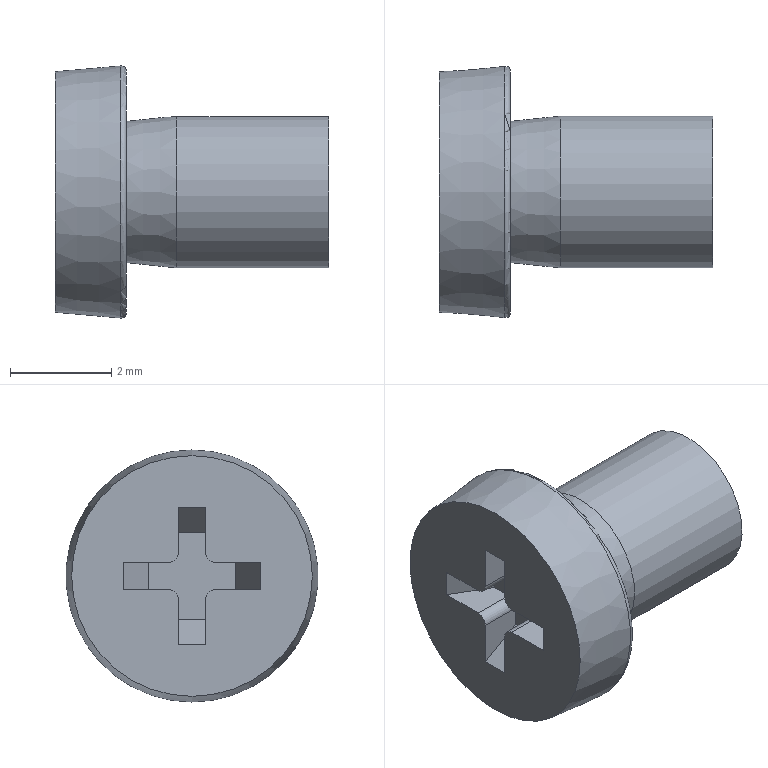Part | STEP file | cross recessed cheese head screws type a gb_GB_CROSS_SCREWS_TYPE135 M3X4-N | 1 solid | 24 faces | box 5.4 x 4.982 x 4.982 mm | volume 52.121 mm3 | plane 16 | cylinder 5 | cone 2 | torus 1 | commonest cylinder face diameters 0.4 x4 3 x1